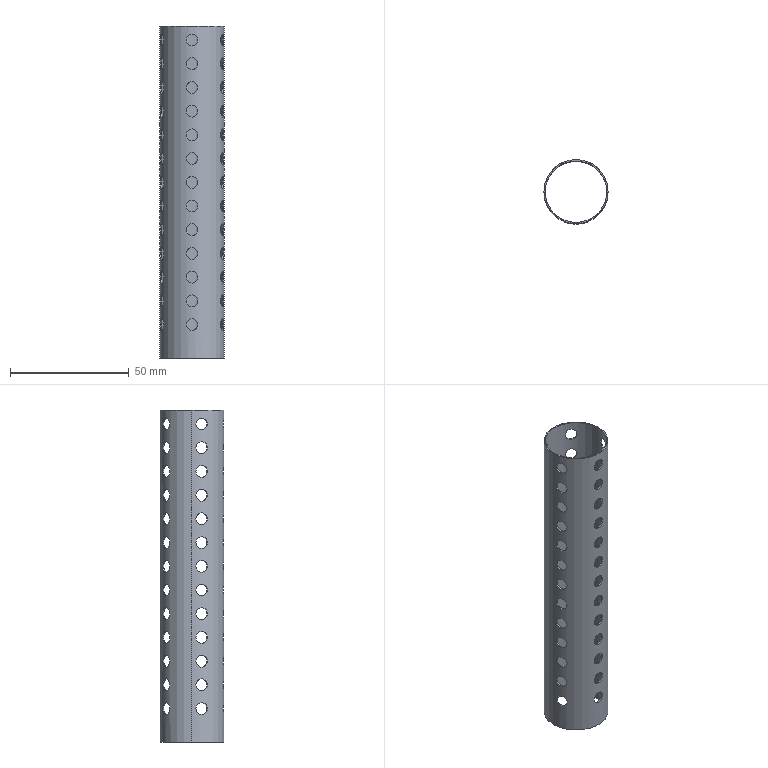Part | SolidWorks | features BaseBody 1 | 1 solid | 136 faces | box 27 x 27 x 140 mm | volume 5187 mm3 | cylinder 134 | plane 2 | commonest cylinder face diameters 5 x130 26 x2 27 x2